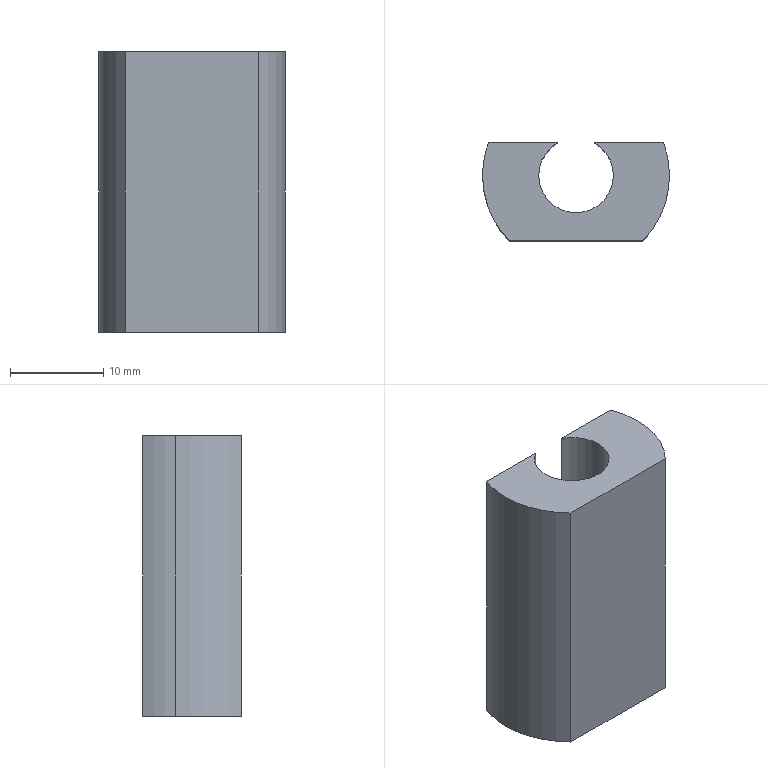Part | STEP file | 001-011-Blanking flip guide rod stopper | 1 solid | 11 faces | box 20 x 10.5 x 30 mm | volume 4413 mm3 | cylinder 6 | plane 5 | commonest cylinder face diameters 8 x3 20 x3
STEP:
#1=CARTESIAN_POINT('',(0.,0.,0.));
#2=DIRECTION('',(0.,0.,1.));
#3=DIRECTION('',(1.,0.,0.));
#4=AXIS2_PLACEMENT_3D('',#1,#2,#3);
#5=CARTESIAN_POINT('',(-4.,0.,30.));
#6=VERTEX_POINT('',#5);
#7=CARTESIAN_POINT('',(-4.,0.,0.));
#8=VERTEX_POINT('',#7);
#9=CARTESIAN_POINT('',(-4.,0.,30.));
#10=DIRECTION('',(0.,0.,-1.));
#11=VECTOR('',#10,1.);
#12=LINE('',#9,#11);
#13=CARTESIAN_POINT('',(0.,0.,30.));
#14=DIRECTION('',(0.,0.,-1.));
#15=DIRECTION('',(-1.,0.,0.));
#16=AXIS2_PLACEMENT_3D('',#13,#14,#15);
#17=CYLINDRICAL_SURFACE('',#16,4.);
#18=CARTESIAN_POINT('',(6.283,0.));
#19=DIRECTION('',(0.,1.));
#20=VECTOR('',#19,1.);
#21=LINE('',#18,#20);
#22=(GEOMETRIC_REPRESENTATION_CONTEXT(2)PARAMETRIC_REPRESENTATION_CONTEXT()REPRESENTATION_CONTEXT('',''));
#23=DEFINITIONAL_REPRESENTATION('',(#21),#22);
#24=PCURVE('',#17,#23);
#25=CARTESIAN_POINT('',(0.,0.,30.));
#26=DIRECTION('',(0.,0.,-1.));
#27=DIRECTION('',(-1.,0.,0.));
#28=AXIS2_PLACEMENT_3D('',#25,#26,#27);
#29=CYLINDRICAL_SURFACE('',#28,4.);
#30=CARTESIAN_POINT('',(0.,0.));
#31=DIRECTION('',(0.,1.));
#32=VECTOR('',#31,1.);
#33=LINE('',#30,#32);
#34=(GEOMETRIC_REPRESENTATION_CONTEXT(2)PARAMETRIC_REPRESENTATION_CONTEXT()REPRESENTATION_CONTEXT('',''));
#35=DEFINITIONAL_REPRESENTATION('',(#33),#34);
#36=PCURVE('',#29,#35);
#37=SURFACE_CURVE('',#12,(#24,#36),.PCURVE_S1.);
#38=EDGE_CURVE('',#6,#8,#37,.T.);
#39=ORIENTED_EDGE('',*,*,#38,.T.);
#40=CARTESIAN_POINT('',(4.,0.,0.));
#41=VERTEX_POINT('',#40);
#42=CARTESIAN_POINT('',(0.,0.,0.));
#43=DIRECTION('',(0.,0.,1.));
#44=DIRECTION('',(1.,0.,0.));
#45=AXIS2_PLACEMENT_3D('',#42,#43,#44);
#46=CIRCLE('',#45,4.);
#47=CARTESIAN_POINT('',(9.425,30.));
#48=DIRECTION('',(-1.,0.));
#49=VECTOR('',#48,1.);
#50=LINE('',#47,#49);
#51=(GEOMETRIC_REPRESENTATION_CONTEXT(2)PARAMETRIC_REPRESENTATION_CONTEXT()REPRESENTATION_CONTEXT('',''));
#52=DEFINITIONAL_REPRESENTATION('',(#50),#51);
#53=PCURVE('',#17,#52);
#54=CARTESIAN_POINT('',(0.,0.,0.));
#55=DIRECTION('',(0.,0.,1.));
#56=DIRECTION('',(1.,0.,0.));
#57=AXIS2_PLACEMENT_3D('',#54,#55,#56);
#58=PLANE('',#57);
#59=CARTESIAN_POINT('',(0.,0.));
#60=DIRECTION('',(1.,0.));
#61=AXIS2_PLACEMENT_2D('',#59,#60);
#62=CIRCLE('',#61,4.);
#63=(GEOMETRIC_REPRESENTATION_CONTEXT(2)PARAMETRIC_REPRESENTATION_CONTEXT()REPRESENTATION_CONTEXT('',''));
#64=DEFINITIONAL_REPRESENTATION('',(#62),#63);
#65=PCURVE('',#58,#64);
#66=SURFACE_CURVE('',#46,(#53,#65),.PCURVE_S1.);
#67=EDGE_CURVE('',#8,#41,#66,.T.);
#68=ORIENTED_EDGE('',*,*,#67,.T.);
#69=CARTESIAN_POINT('',(4.,0.,30.));
#70=VERTEX_POINT('',#69);
#71=CARTESIAN_POINT('',(4.,0.,30.));
#72=DIRECTION('',(0.,0.,-1.));
#73=VECTOR('',#72,1.);
#74=LINE('',#71,#73);
#75=CARTESIAN_POINT('',(3.142,0.));
#76=DIRECTION('',(0.,1.));
#77=VECTOR('',#76,1.);
#78=LINE('',#75,#77);
#79=(GEOMETRIC_REPRESENTATION_CONTEXT(2)PARAMETRIC_REPRESENTATION_CONTEXT()REPRESENTATION_CONTEXT('',''));
#80=DEFINITIONAL_REPRESENTATION('',(#78),#79);
#81=PCURVE('',#17,#80);
#82=CARTESIAN_POINT('',(0.,0.,30.));
#83=DIRECTION('',(0.,0.,-1.));
#84=DIRECTION('',(-1.,0.,0.));
#85=AXIS2_PLACEMENT_3D('',#82,#83,#84);
#86=CYLINDRICAL_SURFACE('',#85,4.);
#87=CARTESIAN_POINT('',(3.142,0.));
#88=DIRECTION('',(0.,1.));
#89=VECTOR('',#88,1.);
#90=LINE('',#87,#89);
#91=(GEOMETRIC_REPRESENTATION_CONTEXT(2)PARAMETRIC_REPRESENTATION_CONTEXT()REPRESENTATION_CONTEXT('',''));
#92=DEFINITIONAL_REPRESENTATION('',(#90),#91);
#93=PCURVE('',#86,#92);
#94=SURFACE_CURVE('',#74,(#81,#93),.PCURVE_S1.);
#95=EDGE_CURVE('',#70,#41,#94,.T.);
#96=ORIENTED_EDGE('',*,*,#95,.F.);
#97=CARTESIAN_POINT('',(0.,0.,30.));
#98=DIRECTION('',(0.,0.,1.));
#99=DIRECTION('',(1.,0.,0.));
#100=AXIS2_PLACEMENT_3D('',#97,#98,#99);
#101=CIRCLE('',#100,4.);
#102=CARTESIAN_POINT('',(9.425,0.));
#103=DIRECTION('',(-1.,0.));
#104=VECTOR('',#103,1.);
#105=LINE('',#102,#104);
#106=(GEOMETRIC_REPRESENTATION_CONTEXT(2)PARAMETRIC_REPRESENTATION_CONTEXT()REPRESENTATION_CONTEXT('',''));
#107=DEFINITIONAL_REPRESENTATION('',(#105),#106);
#108=PCURVE('',#17,#107);
#109=CARTESIAN_POINT('',(0.,0.,30.));
#110=DIRECTION('',(0.,0.,1.));
#111=DIRECTION('',(1.,0.,0.));
#112=AXIS2_PLACEMENT_3D('',#109,#110,#111);
#113=PLANE('',#112);
#114=CARTESIAN_POINT('',(0.,0.));
#115=DIRECTION('',(1.,0.));
#116=AXIS2_PLACEMENT_2D('',#114,#115);
#117=CIRCLE('',#116,4.);
#118=(GEOMETRIC_REPRESENTATION_CONTEXT(2)PARAMETRIC_REPRESENTATION_CONTEXT()REPRESENTATION_CONTEXT('',''));
#119=DEFINITIONAL_REPRESENTATION('',(#117),#118);
#120=PCURVE('',#113,#119);
#121=SURFACE_CURVE('',#101,(#108,#120),.PCURVE_S1.);
#122=EDGE_CURVE('',#6,#70,#121,.T.);
#123=ORIENTED_EDGE('',*,*,#122,.F.);
#124=EDGE_LOOP('',(#39,#68,#96,#123));
#125=FACE_BOUND('',#124,.F.);
#126=ADVANCED_FACE('',(#125),#17,.F.);
#127=CARTESIAN_POINT('',(-1.936,3.5,30.));
#128=VERTEX_POINT('',#127);
#129=CARTESIAN_POINT('',(-1.936,3.5,0.));
#130=VERTEX_POINT('',#129);
#131=CARTESIAN_POINT('',(-1.936,3.5,30.));
#132=DIRECTION('',(0.,0.,-1.));
#133=VECTOR('',#132,1.);
#134=LINE('',#131,#133);
#135=CARTESIAN_POINT('',(1.065,0.));
#136=DIRECTION('',(0.,1.));
#137=VECTOR('',#136,1.);
#138=LINE('',#135,#137);
#139=(GEOMETRIC_REPRESENTATION_CONTEXT(2)PARAMETRIC_REPRESENTATION_CONTEXT()REPRESENTATION_CONTEXT('',''));
#140=DEFINITIONAL_REPRESENTATION('',(#138),#139);
#141=PCURVE('',#29,#140);
#142=CARTESIAN_POINT('',(-10.,3.5,0.));
#143=DIRECTION('',(0.,-1.,0.));
#144=DIRECTION('',(0.,0.,-1.));
#145=AXIS2_PLACEMENT_3D('',#142,#143,#144);
#146=PLANE('',#145);
#147=CARTESIAN_POINT('',(-30.,8.064));
#148=DIRECTION('',(1.,0.));
#149=VECTOR('',#148,1.);
#150=LINE('',#147,#149);
#151=(GEOMETRIC_REPRESENTATION_CONTEXT(2)PARAMETRIC_REPRESENTATION_CONTEXT()REPRESENTATION_CONTEXT('',''));
#152=DEFINITIONAL_REPRESENTATION('',(#150),#151);
#153=PCURVE('',#146,#152);
#154=SURFACE_CURVE('',#134,(#141,#153),.PCURVE_S1.);
#155=EDGE_CURVE('',#128,#130,#154,.T.);
#156=ORIENTED_EDGE('',*,*,#155,.T.);
#157=CARTESIAN_POINT('',(0.,0.,0.));
#158=DIRECTION('',(0.,0.,1.));
#159=DIRECTION('',(1.,0.,0.));
#160=AXIS2_PLACEMENT_3D('',#157,#158,#159);
#161=CIRCLE('',#160,4.);
#162=CARTESIAN_POINT('',(3.142,30.));
#163=DIRECTION('',(-1.,0.));
#164=VECTOR('',#163,1.);
#165=LINE('',#162,#164);
#166=(GEOMETRIC_REPRESENTATION_CONTEXT(2)PARAMETRIC_REPRESENTATION_CONTEXT()REPRESENTATION_CONTEXT('',''));
#167=DEFINITIONAL_REPRESENTATION('',(#165),#166);
#168=PCURVE('',#29,#167);
#169=CARTESIAN_POINT('',(0.,0.));
#170=DIRECTION('',(1.,0.));
#171=AXIS2_PLACEMENT_2D('',#169,#170);
#172=CIRCLE('',#171,4.);
#173=(GEOMETRIC_REPRESENTATION_CONTEXT(2)PARAMETRIC_REPRESENTATION_CONTEXT()REPRESENTATION_CONTEXT('',''));
#174=DEFINITIONAL_REPRESENTATION('',(#172),#173);
#175=PCURVE('',#58,#174);
#176=SURFACE_CURVE('',#161,(#168,#175),.PCURVE_S1.);
#177=EDGE_CURVE('',#130,#8,#176,.T.);
#178=ORIENTED_EDGE('',*,*,#177,.T.);
#179=ORIENTED_EDGE('',*,*,#38,.F.);
#180=CARTESIAN_POINT('',(0.,0.,30.));
#181=DIRECTION('',(0.,0.,1.));
#182=DIRECTION('',(1.,0.,0.));
#183=AXIS2_PLACEMENT_3D('',#180,#181,#182);
#184=CIRCLE('',#183,4.);
#185=CARTESIAN_POINT('',(3.142,0.));
#186=DIRECTION('',(-1.,0.));
#187=VECTOR('',#186,1.);
#188=LINE('',#185,#187);
#189=(GEOMETRIC_REPRESENTATION_CONTEXT(2)PARAMETRIC_REPRESENTATION_CONTEXT()REPRESENTATION_CONTEXT('',''));
#190=DEFINITIONAL_REPRESENTATION('',(#188),#189);
#191=PCURVE('',#29,#190);
#192=CARTESIAN_POINT('',(0.,0.));
#193=DIRECTION('',(1.,0.));
#194=AXIS2_PLACEMENT_2D('',#192,#193);
#195=CIRCLE('',#194,4.);
#196=(GEOMETRIC_REPRESENTATION_CONTEXT(2)PARAMETRIC_REPRESENTATION_CONTEXT()REPRESENTATION_CONTEXT('',''));
#197=DEFINITIONAL_REPRESENTATION('',(#195),#196);
#198=PCURVE('',#113,#197);
#199=SURFACE_CURVE('',#184,(#191,#198),.PCURVE_S1.);
#200=EDGE_CURVE('',#128,#6,#199,.T.);
#201=ORIENTED_EDGE('',*,*,#200,.F.);
#202=EDGE_LOOP('',(#156,#178,#179,#201));
#203=FACE_BOUND('',#202,.F.);
#204=ADVANCED_FACE('',(#203),#29,.F.);
#205=CARTESIAN_POINT('',(-10.,0.,30.));
#206=VERTEX_POINT('',#205);
#207=CARTESIAN_POINT('',(-7.141,-7.,30.));
#208=VERTEX_POINT('',#207);
#209=CARTESIAN_POINT('',(0.,0.,30.));
#210=DIRECTION('',(0.,0.,1.));
#211=DIRECTION('',(1.,0.,0.));
#212=AXIS2_PLACEMENT_3D('',#209,#210,#211);
#213=CIRCLE('',#212,10.);
#214=CARTESIAN_POINT('',(0.,0.,30.));
#215=DIRECTION('',(0.,0.,-1.));
#216=DIRECTION('',(-1.,0.,0.));
#217=AXIS2_PLACEMENT_3D('',#214,#215,#216);
#218=CYLINDRICAL_SURFACE('',#217,10.);
#219=CARTESIAN_POINT('',(9.425,0.));
#220=DIRECTION('',(-1.,0.));
#221=VECTOR('',#220,1.);
#222=LINE('',#219,#221);
#223=(GEOMETRIC_REPRESENTATION_CONTEXT(2)PARAMETRIC_REPRESENTATION_CONTEXT()REPRESENTATION_CONTEXT('',''));
#224=DEFINITIONAL_REPRESENTATION('',(#222),#223);
#225=PCURVE('',#218,#224);
#226=CARTESIAN_POINT('',(0.,0.));
#227=DIRECTION('',(1.,0.));
#228=AXIS2_PLACEMENT_2D('',#226,#227);
#229=CIRCLE('',#228,10.);
#230=(GEOMETRIC_REPRESENTATION_CONTEXT(2)PARAMETRIC_REPRESENTATION_CONTEXT()REPRESENTATION_CONTEXT('',''));
#231=DEFINITIONAL_REPRESENTATION('',(#229),#230);
#232=PCURVE('',#113,#231);
#233=SURFACE_CURVE('',#213,(#225,#232),.PCURVE_S1.);
#234=EDGE_CURVE('',#206,#208,#233,.T.);
#235=ORIENTED_EDGE('',*,*,#234,.F.);
#236=CARTESIAN_POINT('',(-10.,0.,0.));
#237=VERTEX_POINT('',#236);
#238=CARTESIAN_POINT('',(-10.,0.,30.));
#239=DIRECTION('',(0.,0.,-1.));
#240=VECTOR('',#239,1.);
#241=LINE('',#238,#240);
#242=CARTESIAN_POINT('',(6.283,0.));
#243=DIRECTION('',(0.,1.));
#244=VECTOR('',#243,1.);
#245=LINE('',#242,#244);
#246=(GEOMETRIC_REPRESENTATION_CONTEXT(2)PARAMETRIC_REPRESENTATION_CONTEXT()REPRESENTATION_CONTEXT('',''));
#247=DEFINITIONAL_REPRESENTATION('',(#245),#246);
#248=PCURVE('',#218,#247);
#249=CARTESIAN_POINT('',(0.,0.,30.));
#250=DIRECTION('',(0.,0.,-1.));
#251=DIRECTION('',(-1.,0.,0.));
#252=AXIS2_PLACEMENT_3D('',#249,#250,#251);
#253=CYLINDRICAL_SURFACE('',#252,10.);
#254=CARTESIAN_POINT('',(0.,0.));
#255=DIRECTION('',(0.,1.));
#256=VECTOR('',#255,1.);
#257=LINE('',#254,#256);
#258=(GEOMETRIC_REPRESENTATION_CONTEXT(2)PARAMETRIC_REPRESENTATION_CONTEXT()REPRESENTATION_CONTEXT('',''));
#259=DEFINITIONAL_REPRESENTATION('',(#257),#258);
#260=PCURVE('',#253,#259);
#261=SURFACE_CURVE('',#241,(#248,#260),.PCURVE_S1.);
#262=EDGE_CURVE('',#206,#237,#261,.T.);
#263=ORIENTED_EDGE('',*,*,#262,.T.);
#264=CARTESIAN_POINT('',(-7.141,-7.,0.));
#265=VERTEX_POINT('',#264);
#266=CARTESIAN_POINT('',(0.,0.,0.));
#267=DIRECTION('',(0.,0.,1.));
#268=DIRECTION('',(1.,0.,0.));
#269=AXIS2_PLACEMENT_3D('',#266,#267,#268);
#270=CIRCLE('',#269,10.);
#271=CARTESIAN_POINT('',(9.425,30.));
#272=DIRECTION('',(-1.,0.));
#273=VECTOR('',#272,1.);
#274=LINE('',#271,#273);
#275=(GEOMETRIC_REPRESENTATION_CONTEXT(2)PARAMETRIC_REPRESENTATION_CONTEXT()REPRESENTATION_CONTEXT('',''));
#276=DEFINITIONAL_REPRESENTATION('',(#274),#275);
#277=PCURVE('',#218,#276);
#278=CARTESIAN_POINT('',(0.,0.));
#279=DIRECTION('',(1.,0.));
#280=AXIS2_PLACEMENT_2D('',#278,#279);
#281=CIRCLE('',#280,10.);
#282=(GEOMETRIC_REPRESENTATION_CONTEXT(2)PARAMETRIC_REPRESENTATION_CONTEXT()REPRESENTATION_CONTEXT('',''));
#283=DEFINITIONAL_REPRESENTATION('',(#281),#282);
#284=PCURVE('',#58,#283);
#285=SURFACE_CURVE('',#270,(#277,#284),.PCURVE_S1.);
#286=EDGE_CURVE('',#237,#265,#285,.T.);
#287=ORIENTED_EDGE('',*,*,#286,.T.);
#288=CARTESIAN_POINT('',(-7.141,-7.,30.));
#289=DIRECTION('',(0.,0.,-1.));
#290=VECTOR('',#289,1.);
#291=LINE('',#288,#290);
#292=CARTESIAN_POINT('',(5.508,0.));
#293=DIRECTION('',(0.,1.));
#294=VECTOR('',#293,1.);
#295=LINE('',#292,#294);
#296=(GEOMETRIC_REPRESENTATION_CONTEXT(2)PARAMETRIC_REPRESENTATION_CONTEXT()REPRESENTATION_CONTEXT('',''));
#297=DEFINITIONAL_REPRESENTATION('',(#295),#296);
#298=PCURVE('',#218,#297);
#299=CARTESIAN_POINT('',(-15.,-7.,0.));
#300=DIRECTION('',(0.,-1.,0.));
#301=DIRECTION('',(0.,0.,-1.));
#302=AXIS2_PLACEMENT_3D('',#299,#300,#301);
#303=PLANE('',#302);
#304=CARTESIAN_POINT('',(-30.,7.859));
#305=DIRECTION('',(1.,0.));
#306=VECTOR('',#305,1.);
#307=LINE('',#304,#306);
#308=(GEOMETRIC_REPRESENTATION_CONTEXT(2)PARAMETRIC_REPRESENTATION_CONTEXT()REPRESENTATION_CONTEXT('',''));
#309=DEFINITIONAL_REPRESENTATION('',(#307),#308);
#310=PCURVE('',#303,#309);
#311=SURFACE_CURVE('',#291,(#298,#310),.PCURVE_S1.);
#312=EDGE_CURVE('',#208,#265,#311,.T.);
#313=ORIENTED_EDGE('',*,*,#312,.F.);
#314=EDGE_LOOP('',(#235,#263,#287,#313));
#315=FACE_BOUND('',#314,.T.);
#316=ADVANCED_FACE('',(#315),#218,.T.);
#317=CARTESIAN_POINT('',(-9.367,3.5,30.));
#318=VERTEX_POINT('',#317);
#319=CARTESIAN_POINT('',(0.,3.5,30.));
#320=DIRECTION('',(1.,0.,0.));
#321=VECTOR('',#320,1.);
#322=LINE('',#319,#321);
#323=CARTESIAN_POINT('',(0.,3.5));
#324=DIRECTION('',(1.,0.));
#325=VECTOR('',#324,1.);
#326=LINE('',#323,#325);
#327=(GEOMETRIC_REPRESENTATION_CONTEXT(2)PARAMETRIC_REPRESENTATION_CONTEXT()REPRESENTATION_CONTEXT('',''));
#328=DEFINITIONAL_REPRESENTATION('',(#326),#327);
#329=PCURVE('',#113,#328);
#330=CARTESIAN_POINT('',(-30.,10.));
#331=DIRECTION('',(0.,1.));
#332=VECTOR('',#331,1.);
#333=LINE('',#330,#332);
#334=(GEOMETRIC_REPRESENTATION_CONTEXT(2)PARAMETRIC_REPRESENTATION_CONTEXT()REPRESENTATION_CONTEXT('',''));
#335=DEFINITIONAL_REPRESENTATION('',(#333),#334);
#336=PCURVE('',#146,#335);
#337=SURFACE_CURVE('',#322,(#329,#336),.PCURVE_S1.);
#338=EDGE_CURVE('',#318,#128,#337,.T.);
#339=ORIENTED_EDGE('',*,*,#338,.F.);
#340=CARTESIAN_POINT('',(0.,0.,30.));
#341=DIRECTION('',(0.,0.,1.));
#342=DIRECTION('',(1.,0.,0.));
#343=AXIS2_PLACEMENT_3D('',#340,#341,#342);
#344=CIRCLE('',#343,10.);
#345=CARTESIAN_POINT('',(0.,0.));
#346=DIRECTION('',(1.,0.));
#347=AXIS2_PLACEMENT_2D('',#345,#346);
#348=CIRCLE('',#347,10.);
#349=(GEOMETRIC_REPRESENTATION_CONTEXT(2)PARAMETRIC_REPRESENTATION_CONTEXT()REPRESENTATION_CONTEXT('',''));
#350=DEFINITIONAL_REPRESENTATION('',(#348),#349);
#351=PCURVE('',#113,#350);
#352=CARTESIAN_POINT('',(3.142,0.));
#353=DIRECTION('',(-1.,0.));
#354=VECTOR('',#353,1.);
#355=LINE('',#352,#354);
#356=(GEOMETRIC_REPRESENTATION_CONTEXT(2)PARAMETRIC_REPRESENTATION_CONTEXT()REPRESENTATION_CONTEXT('',''));
#357=DEFINITIONAL_REPRESENTATION('',(#355),#356);
#358=PCURVE('',#253,#357);
#359=SURFACE_CURVE('',#344,(#351,#358),.PCURVE_S1.);
#360=EDGE_CURVE('',#318,#206,#359,.T.);
#361=ORIENTED_EDGE('',*,*,#360,.T.);
#362=ORIENTED_EDGE('',*,*,#234,.T.);
#363=CARTESIAN_POINT('',(7.141,-7.,30.));
#364=VERTEX_POINT('',#363);
#365=CARTESIAN_POINT('',(0.,-7.,30.));
#366=DIRECTION('',(1.,0.,0.));
#367=VECTOR('',#366,1.);
#368=LINE('',#365,#367);
#369=CARTESIAN_POINT('',(0.,-7.));
#370=DIRECTION('',(1.,0.));
#371=VECTOR('',#370,1.);
#372=LINE('',#369,#371);
#373=(GEOMETRIC_REPRESENTATION_CONTEXT(2)PARAMETRIC_REPRESENTATION_CONTEXT()REPRESENTATION_CONTEXT('',''));
#374=DEFINITIONAL_REPRESENTATION('',(#372),#373);
#375=PCURVE('',#113,#374);
#376=CARTESIAN_POINT('',(-30.,15.));
#377=DIRECTION('',(0.,1.));
#378=VECTOR('',#377,1.);
#379=LINE('',#376,#378);
#380=(GEOMETRIC_REPRESENTATION_CONTEXT(2)PARAMETRIC_REPRESENTATION_CONTEXT()REPRESENTATION_CONTEXT('',''));
#381=DEFINITIONAL_REPRESENTATION('',(#379),#380);
#382=PCURVE('',#303,#381);
#383=SURFACE_CURVE('',#368,(#375,#382),.PCURVE_S1.);
#384=EDGE_CURVE('',#208,#364,#383,.T.);
#385=ORIENTED_EDGE('',*,*,#384,.T.);
#386=CARTESIAN_POINT('',(9.367,3.5,30.));
#387=VERTEX_POINT('',#386);
#388=CARTESIAN_POINT('',(0.,0.,30.));
#389=DIRECTION('',(0.,0.,1.));
#390=DIRECTION('',(1.,0.,0.));
#391=AXIS2_PLACEMENT_3D('',#388,#389,#390);
#392=CIRCLE('',#391,10.);
#393=CARTESIAN_POINT('',(0.,0.));
#394=DIRECTION('',(1.,0.));
#395=AXIS2_PLACEMENT_2D('',#393,#394);
#396=CIRCLE('',#395,10.);
#397=(GEOMETRIC_REPRESENTATION_CONTEXT(2)PARAMETRIC_REPRESENTATION_CONTEXT()REPRESENTATION_CONTEXT('',''));
#398=DEFINITIONAL_REPRESENTATION('',(#396),#397);
#399=PCURVE('',#113,#398);
#400=CARTESIAN_POINT('',(0.,0.,30.));
#401=DIRECTION('',(0.,0.,-1.));
#402=DIRECTION('',(-1.,0.,0.));
#403=AXIS2_PLACEMENT_3D('',#400,#401,#402);
#404=CYLINDRICAL_SURFACE('',#403,10.);
#405=CARTESIAN_POINT('',(9.425,0.));
#406=DIRECTION('',(-1.,0.));
#407=VECTOR('',#406,1.);
#408=LINE('',#405,#407);
#409=(GEOMETRIC_REPRESENTATION_CONTEXT(2)PARAMETRIC_REPRESENTATION_CONTEXT()REPRESENTATION_CONTEXT('',''));
#410=DEFINITIONAL_REPRESENTATION('',(#408),#409);
#411=PCURVE('',#404,#410);
#412=SURFACE_CURVE('',#392,(#399,#411),.PCURVE_S1.);
#413=EDGE_CURVE('',#364,#387,#412,.T.);
#414=ORIENTED_EDGE('',*,*,#413,.T.);
#415=CARTESIAN_POINT('',(1.936,3.5,30.));
#416=VERTEX_POINT('',#415);
#417=CARTESIAN_POINT('',(0.,3.5,30.));
#418=DIRECTION('',(1.,0.,0.));
#419=VECTOR('',#418,1.);
#420=LINE('',#417,#419);
#421=CARTESIAN_POINT('',(0.,3.5));
#422=DIRECTION('',(1.,0.));
#423=VECTOR('',#422,1.);
#424=LINE('',#421,#423);
#425=(GEOMETRIC_REPRESENTATION_CONTEXT(2)PARAMETRIC_REPRESENTATION_CONTEXT()REPRESENTATION_CONTEXT('',''));
#426=DEFINITIONAL_REPRESENTATION('',(#424),#425);
#427=PCURVE('',#113,#426);
#428=CARTESIAN_POINT('',(-10.,3.5,0.));
#429=DIRECTION('',(0.,-1.,0.));
#430=DIRECTION('',(0.,0.,-1.));
#431=AXIS2_PLACEMENT_3D('',#428,#429,#430);
#432=PLANE('',#431);
#433=CARTESIAN_POINT('',(-30.,10.));
#434=DIRECTION('',(0.,1.));
#435=VECTOR('',#434,1.);
#436=LINE('',#433,#435);
#437=(GEOMETRIC_REPRESENTATION_CONTEXT(2)PARAMETRIC_REPRESENTATION_CONTEXT()REPRESENTATION_CONTEXT('',''));
#438=DEFINITIONAL_REPRESENTATION('',(#436),#437);
#439=PCURVE('',#432,#438);
#440=SURFACE_CURVE('',#420,(#427,#439),.PCURVE_S1.);
#441=EDGE_CURVE('',#416,#387,#440,.T.);
#442=ORIENTED_EDGE('',*,*,#441,.F.);
#443=CARTESIAN_POINT('',(0.,0.,30.));
#444=DIRECTION('',(0.,0.,1.));
#445=DIRECTION('',(1.,0.,0.));
#446=AXIS2_PLACEMENT_3D('',#443,#444,#445);
#447=CIRCLE('',#446,4.);
#448=CARTESIAN_POINT('',(0.,0.));
#449=DIRECTION('',(1.,0.));
#450=AXIS2_PLACEMENT_2D('',#448,#449);
#451=CIRCLE('',#450,4.);
#452=(GEOMETRIC_REPRESENTATION_CONTEXT(2)PARAMETRIC_REPRESENTATION_CONTEXT()REPRESENTATION_CONTEXT('',''));
#453=DEFINITIONAL_REPRESENTATION('',(#451),#452);
#454=PCURVE('',#113,#453);
#455=CARTESIAN_POINT('',(3.142,0.));
#456=DIRECTION('',(-1.,0.));
#457=VECTOR('',#456,1.);
#458=LINE('',#455,#457);
#459=(GEOMETRIC_REPRESENTATION_CONTEXT(2)PARAMETRIC_REPRESENTATION_CONTEXT()REPRESENTATION_CONTEXT('',''));
#460=DEFINITIONAL_REPRESENTATION('',(#458),#459);
#461=PCURVE('',#86,#460);
#462=SURFACE_CURVE('',#447,(#454,#461),.PCURVE_S1.);
#463=EDGE_CURVE('',#70,#416,#462,.T.);
#464=ORIENTED_EDGE('',*,*,#463,.F.);
#465=ORIENTED_EDGE('',*,*,#122,.F.);
#466=ORIENTED_EDGE('',*,*,#200,.F.);
#467=EDGE_LOOP('',(#339,#361,#362,#385,#414,#442,#464,#465,#466));
#468=FACE_BOUND('',#467,.T.);
#469=ADVANCED_FACE('',(#468),#113,.T.);
#470=CARTESIAN_POINT('',(-9.367,3.5,0.));
#471=VERTEX_POINT('',#470);
#472=CARTESIAN_POINT('',(0.,0.,0.));
#473=DIRECTION('',(0.,0.,1.));
#474=DIRECTION('',(1.,0.,0.));
#475=AXIS2_PLACEMENT_3D('',#472,#473,#474);
#476=CIRCLE('',#475,10.);
#477=CARTESIAN_POINT('',(0.,0.));
#478=DIRECTION('',(1.,0.));
#479=AXIS2_PLACEMENT_2D('',#477,#478);
#480=CIRCLE('',#479,10.);
#481=(GEOMETRIC_REPRESENTATION_CONTEXT(2)PARAMETRIC_REPRESENTATION_CONTEXT()REPRESENTATION_CONTEXT('',''));
#482=DEFINITIONAL_REPRESENTATION('',(#480),#481);
#483=PCURVE('',#58,#482);
#484=CARTESIAN_POINT('',(3.142,30.));
#485=DIRECTION('',(-1.,0.));
#486=VECTOR('',#485,1.);
#487=LINE('',#484,#486);
#488=(GEOMETRIC_REPRESENTATION_CONTEXT(2)PARAMETRIC_REPRESENTATION_CONTEXT()REPRESENTATION_CONTEXT('',''));
#489=DEFINITIONAL_REPRESENTATION('',(#487),#488);
#490=PCURVE('',#253,#489);
#491=SURFACE_CURVE('',#476,(#483,#490),.PCURVE_S1.);
#492=EDGE_CURVE('',#471,#237,#491,.T.);
#493=ORIENTED_EDGE('',*,*,#492,.F.);
#494=CARTESIAN_POINT('',(-10.,3.5,0.));
#495=DIRECTION('',(1.,0.,0.));
#496=VECTOR('',#495,1.);
#497=LINE('',#494,#496);
#498=CARTESIAN_POINT('',(-10.,3.5));
#499=DIRECTION('',(1.,0.));
#500=VECTOR('',#499,1.);
#501=LINE('',#498,#500);
#502=(GEOMETRIC_REPRESENTATION_CONTEXT(2)PARAMETRIC_REPRESENTATION_CONTEXT()REPRESENTATION_CONTEXT('',''));
#503=DEFINITIONAL_REPRESENTATION('',(#501),#502);
#504=PCURVE('',#58,#503);
#505=CARTESIAN_POINT('',(0.,0.));
#506=DIRECTION('',(0.,1.));
#507=VECTOR('',#506,1.);
#508=LINE('',#505,#507);
#509=(GEOMETRIC_REPRESENTATION_CONTEXT(2)PARAMETRIC_REPRESENTATION_CONTEXT()REPRESENTATION_CONTEXT('',''));
#510=DEFINITIONAL_REPRESENTATION('',(#508),#509);
#511=PCURVE('',#146,#510);
#512=SURFACE_CURVE('',#497,(#504,#511),.PCURVE_S1.);
#513=EDGE_CURVE('',#471,#130,#512,.T.);
#514=ORIENTED_EDGE('',*,*,#513,.T.);
#515=ORIENTED_EDGE('',*,*,#177,.T.);
#516=ORIENTED_EDGE('',*,*,#67,.T.);
#517=CARTESIAN_POINT('',(1.936,3.5,0.));
#518=VERTEX_POINT('',#517);
#519=CARTESIAN_POINT('',(0.,0.,0.));
#520=DIRECTION('',(0.,0.,1.));
#521=DIRECTION('',(1.,0.,0.));
#522=AXIS2_PLACEMENT_3D('',#519,#520,#521);
#523=CIRCLE('',#522,4.);
#524=CARTESIAN_POINT('',(0.,0.));
#525=DIRECTION('',(1.,0.));
#526=AXIS2_PLACEMENT_2D('',#524,#525);
#527=CIRCLE('',#526,4.);
#528=(GEOMETRIC_REPRESENTATION_CONTEXT(2)PARAMETRIC_REPRESENTATION_CONTEXT()REPRESENTATION_CONTEXT('',''));
#529=DEFINITIONAL_REPRESENTATION('',(#527),#528);
#530=PCURVE('',#58,#529);
#531=CARTESIAN_POINT('',(3.142,30.));
#532=DIRECTION('',(-1.,0.));
#533=VECTOR('',#532,1.);
#534=LINE('',#531,#533);
#535=(GEOMETRIC_REPRESENTATION_CONTEXT(2)PARAMETRIC_REPRESENTATION_CONTEXT()REPRESENTATION_CONTEXT('',''));
#536=DEFINITIONAL_REPRESENTATION('',(#534),#535);
#537=PCURVE('',#86,#536);
#538=SURFACE_CURVE('',#523,(#530,#537),.PCURVE_S1.);
#539=EDGE_CURVE('',#41,#518,#538,.T.);
#540=ORIENTED_EDGE('',*,*,#539,.T.);
#541=CARTESIAN_POINT('',(9.367,3.5,0.));
#542=VERTEX_POINT('',#541);
#543=CARTESIAN_POINT('',(-10.,3.5,0.));
#544=DIRECTION('',(1.,0.,0.));
#545=VECTOR('',#544,1.);
#546=LINE('',#543,#545);
#547=CARTESIAN_POINT('',(-10.,3.5));
#548=DIRECTION('',(1.,0.));
#549=VECTOR('',#548,1.);
#550=LINE('',#547,#549);
#551=(GEOMETRIC_REPRESENTATION_CONTEXT(2)PARAMETRIC_REPRESENTATION_CONTEXT()REPRESENTATION_CONTEXT('',''));
#552=DEFINITIONAL_REPRESENTATION('',(#550),#551);
#553=PCURVE('',#58,#552);
#554=CARTESIAN_POINT('',(0.,0.));
#555=DIRECTION('',(0.,1.));
#556=VECTOR('',#555,1.);
#557=LINE('',#554,#556);
#558=(GEOMETRIC_REPRESENTATION_CONTEXT(2)PARAMETRIC_REPRESENTATION_CONTEXT()REPRESENTATION_CONTEXT('',''));
#559=DEFINITIONAL_REPRESENTATION('',(#557),#558);
#560=PCURVE('',#432,#559);
#561=SURFACE_CURVE('',#546,(#553,#560),.PCURVE_S1.);
#562=EDGE_CURVE('',#518,#542,#561,.T.);
#563=ORIENTED_EDGE('',*,*,#562,.T.);
#564=CARTESIAN_POINT('',(7.141,-7.,0.));
#565=VERTEX_POINT('',#564);
#566=CARTESIAN_POINT('',(0.,0.,0.));
#567=DIRECTION('',(0.,0.,1.));
#568=DIRECTION('',(1.,0.,0.));
#569=AXIS2_PLACEMENT_3D('',#566,#567,#568);
#570=CIRCLE('',#569,10.);
#571=CARTESIAN_POINT('',(0.,0.));
#572=DIRECTION('',(1.,0.));
#573=AXIS2_PLACEMENT_2D('',#571,#572);
#574=CIRCLE('',#573,10.);
#575=(GEOMETRIC_REPRESENTATION_CONTEXT(2)PARAMETRIC_REPRESENTATION_CONTEXT()REPRESENTATION_CONTEXT('',''));
#576=DEFINITIONAL_REPRESENTATION('',(#574),#575);
#577=PCURVE('',#58,#576);
#578=CARTESIAN_POINT('',(9.425,30.));
#579=DIRECTION('',(-1.,0.));
#580=VECTOR('',#579,1.);
#581=LINE('',#578,#580);
#582=(GEOMETRIC_REPRESENTATION_CONTEXT(2)PARAMETRIC_REPRESENTATION_CONTEXT()REPRESENTATION_CONTEXT('',''));
#583=DEFINITIONAL_REPRESENTATION('',(#581),#582);
#584=PCURVE('',#404,#583);
#585=SURFACE_CURVE('',#570,(#577,#584),.PCURVE_S1.);
#586=EDGE_CURVE('',#565,#542,#585,.T.);
#587=ORIENTED_EDGE('',*,*,#586,.F.);
#588=CARTESIAN_POINT('',(-15.,-7.,0.));
#589=DIRECTION('',(1.,0.,0.));
#590=VECTOR('',#589,1.);
#591=LINE('',#588,#590);
#592=CARTESIAN_POINT('',(-15.,-7.));
#593=DIRECTION('',(1.,0.));
#594=VECTOR('',#593,1.);
#595=LINE('',#592,#594);
#596=(GEOMETRIC_REPRESENTATION_CONTEXT(2)PARAMETRIC_REPRESENTATION_CONTEXT()REPRESENTATION_CONTEXT('',''));
#597=DEFINITIONAL_REPRESENTATION('',(#595),#596);
#598=PCURVE('',#58,#597);
#599=CARTESIAN_POINT('',(0.,0.));
#600=DIRECTION('',(0.,1.));
#601=VECTOR('',#600,1.);
#602=LINE('',#599,#601);
#603=(GEOMETRIC_REPRESENTATION_CONTEXT(2)PARAMETRIC_REPRESENTATION_CONTEXT()REPRESENTATION_CONTEXT('',''));
#604=DEFINITIONAL_REPRESENTATION('',(#602),#603);
#605=PCURVE('',#303,#604);
#606=SURFACE_CURVE('',#591,(#598,#605),.PCURVE_S1.);
#607=EDGE_CURVE('',#265,#565,#606,.T.);
#608=ORIENTED_EDGE('',*,*,#607,.F.);
#609=ORIENTED_EDGE('',*,*,#286,.F.);
#610=EDGE_LOOP('',(#493,#514,#515,#516,#540,#563,#587,#608,#609));
#611=FACE_BOUND('',#610,.T.);
#612=ADVANCED_FACE('',(#611),#58,.F.);
#613=ORIENTED_EDGE('',*,*,#262,.F.);
#614=ORIENTED_EDGE('',*,*,#360,.F.);
#615=CARTESIAN_POINT('',(-9.367,3.5,30.));
#616=DIRECTION('',(0.,0.,-1.));
#617=VECTOR('',#616,1.);
#618=LINE('',#615,#617);
#619=CARTESIAN_POINT('',(0.3576,0.));
#620=DIRECTION('',(0.,1.));
#621=VECTOR('',#620,1.);
#622=LINE('',#619,#621);
#623=(GEOMETRIC_REPRESENTATION_CONTEXT(2)PARAMETRIC_REPRESENTATION_CONTEXT()REPRESENTATION_CONTEXT('',''));
#624=DEFINITIONAL_REPRESENTATION('',(#622),#623);
#625=PCURVE('',#253,#624);
#626=CARTESIAN_POINT('',(-30.,0.6325));
#627=DIRECTION('',(1.,0.));
#628=VECTOR('',#627,1.);
#629=LINE('',#626,#628);
#630=(GEOMETRIC_REPRESENTATION_CONTEXT(2)PARAMETRIC_REPRESENTATION_CONTEXT()REPRESENTATION_CONTEXT('',''));
#631=DEFINITIONAL_REPRESENTATION('',(#629),#630);
#632=PCURVE('',#146,#631);
#633=SURFACE_CURVE('',#618,(#625,#632),.PCURVE_S1.);
#634=EDGE_CURVE('',#318,#471,#633,.T.);
#635=ORIENTED_EDGE('',*,*,#634,.T.);
#636=ORIENTED_EDGE('',*,*,#492,.T.);
#637=EDGE_LOOP('',(#613,#614,#635,#636));
#638=FACE_BOUND('',#637,.T.);
#639=ADVANCED_FACE('',(#638),#253,.T.);
#640=ORIENTED_EDGE('',*,*,#586,.T.);
#641=CARTESIAN_POINT('',(9.367,3.5,30.));
#642=DIRECTION('',(0.,0.,1.));
#643=VECTOR('',#642,1.);
#644=LINE('',#641,#643);
#645=CARTESIAN_POINT('',(2.784,0.));
#646=DIRECTION('',(0.,-1.));
#647=VECTOR('',#646,1.);
#648=LINE('',#645,#647);
#649=(GEOMETRIC_REPRESENTATION_CONTEXT(2)PARAMETRIC_REPRESENTATION_CONTEXT()REPRESENTATION_CONTEXT('',''));
#650=DEFINITIONAL_REPRESENTATION('',(#648),#649);
#651=PCURVE('',#404,#650);
#652=CARTESIAN_POINT('',(-30.,19.367));
#653=DIRECTION('',(-1.,0.));
#654=VECTOR('',#653,1.);
#655=LINE('',#652,#654);
#656=(GEOMETRIC_REPRESENTATION_CONTEXT(2)PARAMETRIC_REPRESENTATION_CONTEXT()REPRESENTATION_CONTEXT('',''));
#657=DEFINITIONAL_REPRESENTATION('',(#655),#656);
#658=PCURVE('',#432,#657);
#659=SURFACE_CURVE('',#644,(#651,#658),.PCURVE_S1.);
#660=EDGE_CURVE('',#542,#387,#659,.T.);
#661=ORIENTED_EDGE('',*,*,#660,.T.);
#662=ORIENTED_EDGE('',*,*,#413,.F.);
#663=CARTESIAN_POINT('',(7.141,-7.,30.));
#664=DIRECTION('',(0.,0.,1.));
#665=VECTOR('',#664,1.);
#666=LINE('',#663,#665);
#667=CARTESIAN_POINT('',(3.917,0.));
#668=DIRECTION('',(0.,-1.));
#669=VECTOR('',#668,1.);
#670=LINE('',#667,#669);
#671=(GEOMETRIC_REPRESENTATION_CONTEXT(2)PARAMETRIC_REPRESENTATION_CONTEXT()REPRESENTATION_CONTEXT('',''));
#672=DEFINITIONAL_REPRESENTATION('',(#670),#671);
#673=PCURVE('',#404,#672);
#674=CARTESIAN_POINT('',(-30.,22.141));
#675=DIRECTION('',(-1.,0.));
#676=VECTOR('',#675,1.);
#677=LINE('',#674,#676);
#678=(GEOMETRIC_REPRESENTATION_CONTEXT(2)PARAMETRIC_REPRESENTATION_CONTEXT()REPRESENTATION_CONTEXT('',''));
#679=DEFINITIONAL_REPRESENTATION('',(#677),#678);
#680=PCURVE('',#303,#679);
#681=SURFACE_CURVE('',#666,(#673,#680),.PCURVE_S1.);
#682=EDGE_CURVE('',#565,#364,#681,.T.);
#683=ORIENTED_EDGE('',*,*,#682,.F.);
#684=EDGE_LOOP('',(#640,#661,#662,#683));
#685=FACE_BOUND('',#684,.T.);
#686=ADVANCED_FACE('',(#685),#404,.T.);
#687=ORIENTED_EDGE('',*,*,#539,.T.);
#688=CARTESIAN_POINT('',(1.936,3.5,30.));
#689=DIRECTION('',(0.,0.,1.));
#690=VECTOR('',#689,1.);
#691=LINE('',#688,#690);
#692=CARTESIAN_POINT('',(2.076,0.));
#693=DIRECTION('',(0.,-1.));
#694=VECTOR('',#693,1.);
#695=LINE('',#692,#694);
#696=(GEOMETRIC_REPRESENTATION_CONTEXT(2)PARAMETRIC_REPRESENTATION_CONTEXT()REPRESENTATION_CONTEXT('',''));
#697=DEFINITIONAL_REPRESENTATION('',(#695),#696);
#698=PCURVE('',#86,#697);
#699=CARTESIAN_POINT('',(-30.,11.936));
#700=DIRECTION('',(-1.,0.));
#701=VECTOR('',#700,1.);
#702=LINE('',#699,#701);
#703=(GEOMETRIC_REPRESENTATION_CONTEXT(2)PARAMETRIC_REPRESENTATION_CONTEXT()REPRESENTATION_CONTEXT('',''));
#704=DEFINITIONAL_REPRESENTATION('',(#702),#703);
#705=PCURVE('',#432,#704);
#706=SURFACE_CURVE('',#691,(#698,#705),.PCURVE_S1.);
#707=EDGE_CURVE('',#518,#416,#706,.T.);
#708=ORIENTED_EDGE('',*,*,#707,.T.);
#709=ORIENTED_EDGE('',*,*,#463,.F.);
#710=ORIENTED_EDGE('',*,*,#95,.T.);
#711=EDGE_LOOP('',(#687,#708,#709,#710));
#712=FACE_BOUND('',#711,.F.);
#713=ADVANCED_FACE('',(#712),#86,.F.);
#714=ORIENTED_EDGE('',*,*,#312,.T.);
#715=ORIENTED_EDGE('',*,*,#607,.T.);
#716=ORIENTED_EDGE('',*,*,#682,.T.);
#717=ORIENTED_EDGE('',*,*,#384,.F.);
#718=EDGE_LOOP('',(#714,#715,#716,#717));
#719=FACE_BOUND('',#718,.T.);
#720=ADVANCED_FACE('',(#719),#303,.T.);
#721=ORIENTED_EDGE('',*,*,#562,.F.);
#722=ORIENTED_EDGE('',*,*,#707,.T.);
#723=ORIENTED_EDGE('',*,*,#441,.T.);
#724=ORIENTED_EDGE('',*,*,#660,.F.);
#725=EDGE_LOOP('',(#721,#722,#723,#724));
#726=FACE_BOUND('',#725,.T.);
#727=ADVANCED_FACE('',(#726),#432,.F.);
#728=ORIENTED_EDGE('',*,*,#338,.T.);
#729=ORIENTED_EDGE('',*,*,#155,.T.);
#730=ORIENTED_EDGE('',*,*,#513,.F.);
#731=ORIENTED_EDGE('',*,*,#634,.F.);
#732=EDGE_LOOP('',(#728,#729,#730,#731));
#733=FACE_BOUND('',#732,.T.);
#734=ADVANCED_FACE('',(#733),#146,.F.);
#735=CLOSED_SHELL('',(#126,#204,#316,#469,#612,#639,#686,#713,#720,#727,#734));
#736=MANIFOLD_SOLID_BREP('',#735);
#737=(LENGTH_UNIT()NAMED_UNIT(*)SI_UNIT(.MILLI.,.METRE.));
#738=UNCERTAINTY_MEASURE_WITH_UNIT(LENGTH_MEASURE(0.0000001),#737,'','');
#739=(NAMED_UNIT(*)PLANE_ANGLE_UNIT()SI_UNIT($,.RADIAN.));
#740=(NAMED_UNIT(*)SI_UNIT($,.STERADIAN.)SOLID_ANGLE_UNIT());
#741=(GEOMETRIC_REPRESENTATION_CONTEXT(3)GLOBAL_UNCERTAINTY_ASSIGNED_CONTEXT((#738))GLOBAL_UNIT_ASSIGNED_CONTEXT((#737,#739,#740))REPRESENTATION_CONTEXT('',''));
#742=ADVANCED_BREP_SHAPE_REPRESENTATION('',(#4,#736),#741);